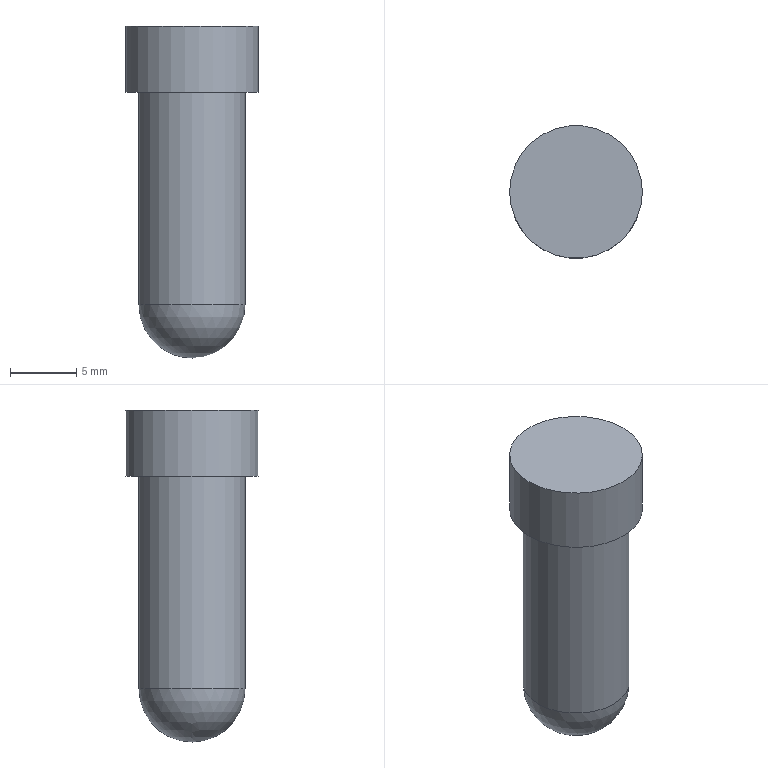Part | NX | features solid 2 | 1 solid | 5 faces | box 10 x 10 x 25 mm | volume 1331 mm3 | cylinder 2 | plane 2 | sphere 1 | commonest cylinder face diameters 8 x1 10 x1
STEP:
#1=CARTESIAN_POINT('',(-626.,-700.,-131.));
#2=VERTEX_POINT('',#1);
#3=CARTESIAN_POINT('',(-630.,-700.,-131.));
#4=DIRECTION('',(0.,0.,1.));
#5=DIRECTION('',(1.,0.,0.));
#6=AXIS2_PLACEMENT_3D('',#3,#4,#5);
#7=CIRCLE('',#6,4.);
#8=EDGE_CURVE('',#2,#2,#7,.T.);
#9=ORIENTED_EDGE('',*,*,#8,.T.);
#10=EDGE_LOOP('',(#9));
#11=FACE_BOUND('',#10,.T.);
#12=CARTESIAN_POINT('',(-634.,-700.,-115.));
#13=VERTEX_POINT('',#12);
#14=CARTESIAN_POINT('',(-630.,-700.,-115.));
#15=DIRECTION('',(0.,0.,-1.));
#16=DIRECTION('',(-1.,0.,0.));
#17=AXIS2_PLACEMENT_3D('',#14,#15,#16);
#18=CIRCLE('',#17,4.);
#19=EDGE_CURVE('',#13,#13,#18,.T.);
#20=ORIENTED_EDGE('',*,*,#19,.T.);
#21=EDGE_LOOP('',(#20));
#22=FACE_BOUND('',#21,.T.);
#23=CARTESIAN_POINT('',(-630.,-700.,-135.));
#24=DIRECTION('',(0.,0.,1.));
#25=DIRECTION('',(1.,0.,0.));
#26=AXIS2_PLACEMENT_3D('',#23,#24,#25);
#27=CYLINDRICAL_SURFACE('',#26,4.);
#28=ADVANCED_FACE('',(#11,#22),#27,.T.);
#29=ORIENTED_EDGE('',*,*,#8,.F.);
#30=EDGE_LOOP('',(#29));
#31=FACE_BOUND('',#30,.T.);
#32=CARTESIAN_POINT('',(-630.,-700.,-131.));
#33=DIRECTION('',(0.,0.,-1.));
#34=DIRECTION('',(-1.,0.,0.));
#35=AXIS2_PLACEMENT_3D('',#32,#33,#34);
#36=SPHERICAL_SURFACE('',#35,4.);
#37=ADVANCED_FACE('',(#31),#36,.T.);
#38=CARTESIAN_POINT('',(-635.,-700.,-115.));
#39=VERTEX_POINT('',#38);
#40=CARTESIAN_POINT('',(-630.,-700.,-115.));
#41=DIRECTION('',(0.,0.,-1.));
#42=DIRECTION('',(-1.,0.,0.));
#43=AXIS2_PLACEMENT_3D('',#40,#41,#42);
#44=CIRCLE('',#43,5.);
#45=EDGE_CURVE('',#39,#39,#44,.T.);
#46=ORIENTED_EDGE('',*,*,#45,.T.);
#47=EDGE_LOOP('',(#46));
#48=FACE_BOUND('',#47,.T.);
#49=ORIENTED_EDGE('',*,*,#19,.F.);
#50=EDGE_LOOP('',(#49));
#51=FACE_BOUND('',#50,.T.);
#52=CARTESIAN_POINT('',(-630.,-700.,-115.));
#53=DIRECTION('',(0.,0.,-1.));
#54=DIRECTION('',(-1.,0.,0.));
#55=AXIS2_PLACEMENT_3D('',#52,#53,#54);
#56=PLANE('',#55);
#57=ADVANCED_FACE('',(#48,#51),#56,.T.);
#58=CARTESIAN_POINT('',(-635.,-700.,-110.));
#59=VERTEX_POINT('',#58);
#60=CARTESIAN_POINT('',(-630.,-700.,-110.));
#61=DIRECTION('',(0.,0.,-1.));
#62=DIRECTION('',(-1.,0.,0.));
#63=AXIS2_PLACEMENT_3D('',#60,#61,#62);
#64=CIRCLE('',#63,5.);
#65=EDGE_CURVE('',#59,#59,#64,.T.);
#66=ORIENTED_EDGE('',*,*,#65,.T.);
#67=EDGE_LOOP('',(#66));
#68=FACE_BOUND('',#67,.T.);
#69=ORIENTED_EDGE('',*,*,#45,.F.);
#70=EDGE_LOOP('',(#69));
#71=FACE_BOUND('',#70,.T.);
#72=CARTESIAN_POINT('',(-630.,-700.,-110.));
#73=DIRECTION('',(0.,0.,-1.));
#74=DIRECTION('',(-1.,0.,0.));
#75=AXIS2_PLACEMENT_3D('',#72,#73,#74);
#76=CYLINDRICAL_SURFACE('',#75,5.);
#77=ADVANCED_FACE('',(#68,#71),#76,.T.);
#78=ORIENTED_EDGE('',*,*,#65,.F.);
#79=EDGE_LOOP('',(#78));
#80=FACE_BOUND('',#79,.T.);
#81=CARTESIAN_POINT('',(-630.,-700.,-110.));
#82=DIRECTION('',(0.,0.,-1.));
#83=DIRECTION('',(-1.,0.,0.));
#84=AXIS2_PLACEMENT_3D('',#81,#82,#83);
#85=PLANE('',#84);
#86=ADVANCED_FACE('',(#80),#85,.F.);
#87=CLOSED_SHELL('',(#28,#37,#57,#77,#86));
#88=MANIFOLD_SOLID_BREP('',#87);
#89=(LENGTH_UNIT()NAMED_UNIT(*)SI_UNIT(.MILLI.,.METRE.));
#90=UNCERTAINTY_MEASURE_WITH_UNIT(LENGTH_MEASURE(0.00001),#89,'','');
#91=(NAMED_UNIT(*)PLANE_ANGLE_UNIT()SI_UNIT($,.RADIAN.));
#92=(NAMED_UNIT(*)SI_UNIT($,.STERADIAN.)SOLID_ANGLE_UNIT());
#93=(GEOMETRIC_REPRESENTATION_CONTEXT(3)GLOBAL_UNCERTAINTY_ASSIGNED_CONTEXT((#90))GLOBAL_UNIT_ASSIGNED_CONTEXT((#89,#91,#92))REPRESENTATION_CONTEXT('',''));
#94=ADVANCED_BREP_SHAPE_REPRESENTATION('',(#88),#93);